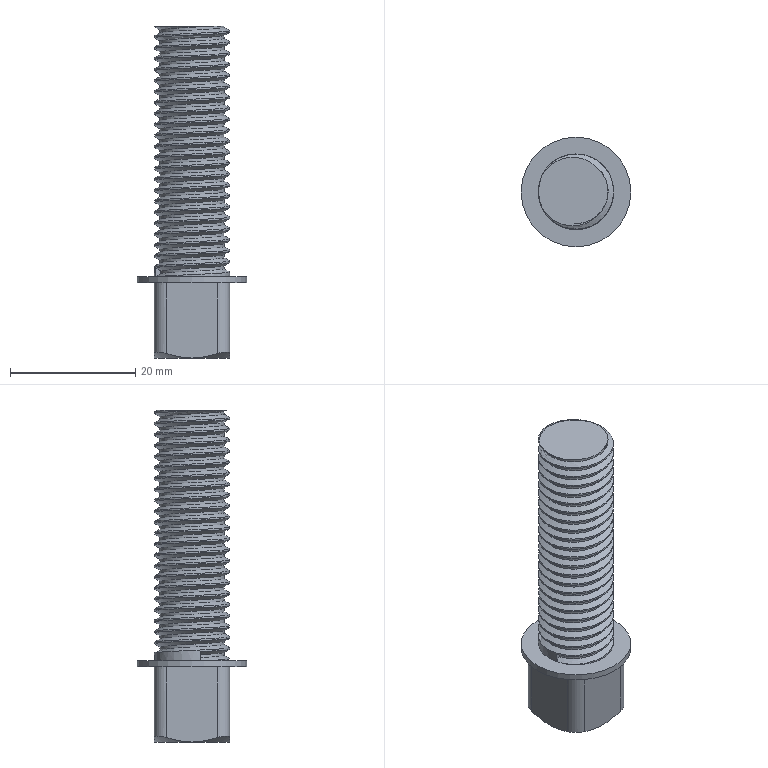Part | NX | features EXTRUDE 4, DATUM_CSYS 2, SKETCH 1, THREADS 1 | 3 solids | 24 faces | box 17.5 x 17.5 x 53 mm | volume 5763 mm3 | plane 11 | cylinder 7 | cone 4 | spline 2 | commonest cylinder face diameters 4 x4 10.25 x1 12 x1 17.5 x1